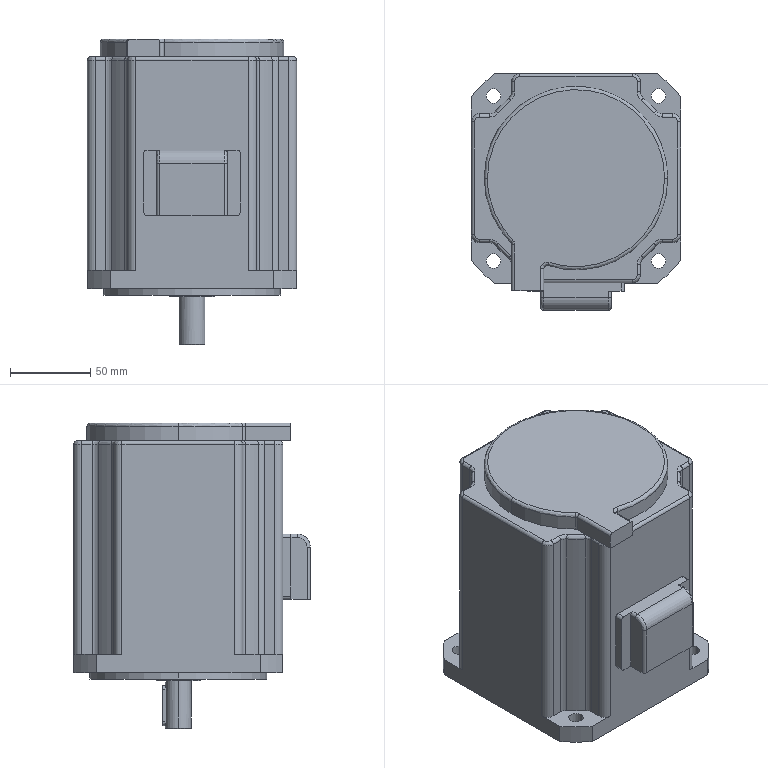Part | STEP file | W-L02641 | 1 solid | 140 faces | box 130 x 147 x 190 mm | volume 2320487 mm3 | cylinder 71 | plane 38 | spline 27 | cone 4 | commonest cylinder face diameters 4 x24 10 x16 9 x8 130 x4 165 x4 5 x3